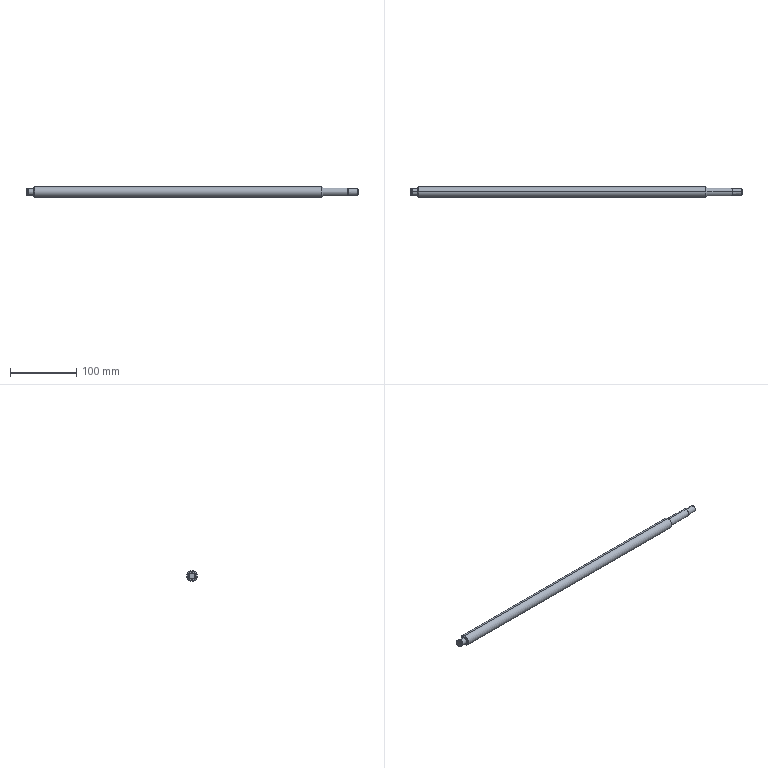Part | SolidWorks | features BaseBody 1, MoveFace 1 | 1 solid | 29 faces | box 500 x 16 x 16 mm | volume 93789 mm3 | cylinder 12 | cone 10 | plane 7 | commonest cylinder face diameters 10 x6 9.6 x2 12 x2 16 x2
STEP:
#1=CARTESIAN_POINT('',(445.773,8.,0.));
#2=VERTEX_POINT('',#1);
#3=CARTESIAN_POINT('',(445.773,0.,-8.));
#4=VERTEX_POINT('',#3);
#5=CARTESIAN_POINT('',(445.773,0.,0.));
#6=DIRECTION('',(-1.,0.,0.));
#7=DIRECTION('',(0.,0.,1.));
#8=AXIS2_PLACEMENT_3D('',#5,#6,#7);
#9=CIRCLE('',#8,8.);
#10=EDGE_CURVE('',#2,#4,#9,.T.);
#11=ORIENTED_EDGE('',*,*,#10,.T.);
#12=CARTESIAN_POINT('',(13.227,0.,-8.));
#13=VERTEX_POINT('',#12);
#14=CARTESIAN_POINT('',(500.,0.,-8.));
#15=DIRECTION('',(-1.,0.,0.));
#16=VECTOR('',#15,1000.);
#17=LINE('',#14,#16);
#18=EDGE_CURVE('',#4,#13,#17,.T.);
#19=ORIENTED_EDGE('',*,*,#18,.T.);
#20=CARTESIAN_POINT('',(13.227,8.,0.));
#21=VERTEX_POINT('',#20);
#22=CARTESIAN_POINT('',(13.227,0.,0.));
#23=DIRECTION('',(1.,0.,0.));
#24=DIRECTION('',(0.,0.,1.));
#25=AXIS2_PLACEMENT_3D('',#22,#23,#24);
#26=CIRCLE('',#25,8.);
#27=EDGE_CURVE('',#13,#21,#26,.T.);
#28=ORIENTED_EDGE('',*,*,#27,.T.);
#29=CARTESIAN_POINT('',(13.227,0.,8.));
#30=VERTEX_POINT('',#29);
#31=CARTESIAN_POINT('',(13.227,0.,0.));
#32=DIRECTION('',(1.,0.,0.));
#33=DIRECTION('',(0.,0.,1.));
#34=AXIS2_PLACEMENT_3D('',#31,#32,#33);
#35=CIRCLE('',#34,8.);
#36=EDGE_CURVE('',#21,#30,#35,.T.);
#37=ORIENTED_EDGE('',*,*,#36,.T.);
#38=CARTESIAN_POINT('',(445.773,0.,8.));
#39=VERTEX_POINT('',#38);
#40=CARTESIAN_POINT('',(500.,0.,8.));
#41=DIRECTION('',(-1.,0.,0.));
#42=VECTOR('',#41,1000.);
#43=LINE('',#40,#42);
#44=EDGE_CURVE('',#39,#30,#43,.T.);
#45=ORIENTED_EDGE('',*,*,#44,.F.);
#46=CARTESIAN_POINT('',(445.773,0.,0.));
#47=DIRECTION('',(-1.,0.,0.));
#48=DIRECTION('',(0.,0.,1.));
#49=AXIS2_PLACEMENT_3D('',#46,#47,#48);
#50=CIRCLE('',#49,8.);
#51=EDGE_CURVE('',#39,#2,#50,.T.);
#52=ORIENTED_EDGE('',*,*,#51,.T.);
#53=EDGE_LOOP('',(#11,#19,#28,#37,#45,#52));
#54=FACE_OUTER_BOUND('',#53,.T.);
#55=CARTESIAN_POINT('',(500.,0.,0.));
#56=DIRECTION('',(-1.,0.,0.));
#57=DIRECTION('',(0.,0.,1.));
#58=AXIS2_PLACEMENT_3D('',#55,#56,#57);
#59=CYLINDRICAL_SURFACE('',#58,8.);
#60=ADVANCED_FACE('',(#54),#59,.T.);
#61=CARTESIAN_POINT('',(12.,6.773,0.));
#62=VERTEX_POINT('',#61);
#63=CARTESIAN_POINT('',(12.,-6.773,0.));
#64=VERTEX_POINT('',#63);
#65=CARTESIAN_POINT('',(12.,0.,0.));
#66=DIRECTION('',(1.,0.,0.));
#67=DIRECTION('',(0.,1.,0.));
#68=AXIS2_PLACEMENT_3D('',#65,#66,#67);
#69=CIRCLE('',#68,6.773);
#70=EDGE_CURVE('',#62,#64,#69,.T.);
#71=ORIENTED_EDGE('',*,*,#70,.T.);
#72=CARTESIAN_POINT('',(13.227,-8.,0.));
#73=VERTEX_POINT('',#72);
#74=CARTESIAN_POINT('',(13.227,-8.,0.));
#75=DIRECTION('',(0.7071,-0.7071,0.));
#76=VECTOR('',#75,1000.);
#77=LINE('',#74,#76);
#78=EDGE_CURVE('',#64,#73,#77,.T.);
#79=ORIENTED_EDGE('',*,*,#78,.T.);
#80=CARTESIAN_POINT('',(13.227,0.,0.));
#81=DIRECTION('',(1.,0.,0.));
#82=DIRECTION('',(0.,0.,1.));
#83=AXIS2_PLACEMENT_3D('',#80,#81,#82);
#84=CIRCLE('',#83,8.);
#85=EDGE_CURVE('',#30,#73,#84,.T.);
#86=ORIENTED_EDGE('',*,*,#85,.F.);
#87=ORIENTED_EDGE('',*,*,#36,.F.);
#88=CARTESIAN_POINT('',(13.227,8.,0.));
#89=DIRECTION('',(0.7071,0.7071,0.));
#90=VECTOR('',#89,1000.);
#91=LINE('',#88,#90);
#92=EDGE_CURVE('',#62,#21,#91,.T.);
#93=ORIENTED_EDGE('',*,*,#92,.F.);
#94=EDGE_LOOP('',(#71,#79,#86,#87,#93));
#95=FACE_OUTER_BOUND('',#94,.T.);
#96=CARTESIAN_POINT('',(13.227,0.,0.));
#97=DIRECTION('',(1.,0.,0.));
#98=DIRECTION('',(0.,1.,0.));
#99=AXIS2_PLACEMENT_3D('',#96,#97,#98);
#100=CONICAL_SURFACE('',#99,8.,0.7854);
#101=ADVANCED_FACE('',(#95),#100,.T.);
#102=CARTESIAN_POINT('',(447.,-6.773,0.));
#103=VERTEX_POINT('',#102);
#104=CARTESIAN_POINT('',(447.,6.773,0.));
#105=VERTEX_POINT('',#104);
#106=CARTESIAN_POINT('',(447.,0.,0.));
#107=DIRECTION('',(-1.,0.,0.));
#108=DIRECTION('',(0.,-1.,0.));
#109=AXIS2_PLACEMENT_3D('',#106,#107,#108);
#110=CIRCLE('',#109,6.773);
#111=EDGE_CURVE('',#103,#105,#110,.T.);
#112=ORIENTED_EDGE('',*,*,#111,.T.);
#113=CARTESIAN_POINT('',(445.773,8.,0.));
#114=DIRECTION('',(-0.7071,0.7071,0.));
#115=VECTOR('',#114,1000.);
#116=LINE('',#113,#115);
#117=EDGE_CURVE('',#105,#2,#116,.T.);
#118=ORIENTED_EDGE('',*,*,#117,.T.);
#119=ORIENTED_EDGE('',*,*,#51,.F.);
#120=CARTESIAN_POINT('',(445.773,-8.,0.));
#121=VERTEX_POINT('',#120);
#122=CARTESIAN_POINT('',(445.773,0.,0.));
#123=DIRECTION('',(-1.,0.,0.));
#124=DIRECTION('',(0.,0.,1.));
#125=AXIS2_PLACEMENT_3D('',#122,#123,#124);
#126=CIRCLE('',#125,8.);
#127=EDGE_CURVE('',#121,#39,#126,.T.);
#128=ORIENTED_EDGE('',*,*,#127,.F.);
#129=CARTESIAN_POINT('',(445.773,-8.,0.));
#130=DIRECTION('',(-0.7071,-0.7071,0.));
#131=VECTOR('',#130,1000.);
#132=LINE('',#129,#131);
#133=EDGE_CURVE('',#103,#121,#132,.T.);
#134=ORIENTED_EDGE('',*,*,#133,.F.);
#135=EDGE_LOOP('',(#112,#118,#119,#128,#134));
#136=FACE_OUTER_BOUND('',#135,.T.);
#137=CARTESIAN_POINT('',(445.773,0.,0.));
#138=DIRECTION('',(-1.,0.,0.));
#139=DIRECTION('',(0.,-1.,0.));
#140=AXIS2_PLACEMENT_3D('',#137,#138,#139);
#141=CONICAL_SURFACE('',#140,8.,0.7854);
#142=ADVANCED_FACE('',(#136),#141,.T.);
#143=CARTESIAN_POINT('',(12.,0.,5.));
#144=VERTEX_POINT('',#143);
#145=CARTESIAN_POINT('',(12.,0.,-5.));
#146=VERTEX_POINT('',#145);
#147=CARTESIAN_POINT('',(12.,0.,0.));
#148=DIRECTION('',(-1.,0.,0.));
#149=DIRECTION('',(0.,0.,1.));
#150=AXIS2_PLACEMENT_3D('',#147,#148,#149);
#151=CIRCLE('',#150,5.);
#152=EDGE_CURVE('',#144,#146,#151,.T.);
#153=ORIENTED_EDGE('',*,*,#152,.T.);
#154=CARTESIAN_POINT('',(4.,0.,-5.));
#155=VERTEX_POINT('',#154);
#156=CARTESIAN_POINT('',(500.,0.,-5.));
#157=DIRECTION('',(-1.,0.,0.));
#158=VECTOR('',#157,1000.);
#159=LINE('',#156,#158);
#160=EDGE_CURVE('',#146,#155,#159,.T.);
#161=ORIENTED_EDGE('',*,*,#160,.T.);
#162=CARTESIAN_POINT('',(4.,0.,5.));
#163=VERTEX_POINT('',#162);
#164=CARTESIAN_POINT('',(4.,0.,0.));
#165=DIRECTION('',(1.,0.,0.));
#166=DIRECTION('',(0.,0.,1.));
#167=AXIS2_PLACEMENT_3D('',#164,#165,#166);
#168=CIRCLE('',#167,5.);
#169=EDGE_CURVE('',#155,#163,#168,.T.);
#170=ORIENTED_EDGE('',*,*,#169,.T.);
#171=CARTESIAN_POINT('',(500.,0.,5.));
#172=DIRECTION('',(-1.,0.,0.));
#173=VECTOR('',#172,1000.);
#174=LINE('',#171,#173);
#175=EDGE_CURVE('',#144,#163,#174,.T.);
#176=ORIENTED_EDGE('',*,*,#175,.F.);
#177=EDGE_LOOP('',(#153,#161,#170,#176));
#178=FACE_OUTER_BOUND('',#177,.T.);
#179=CARTESIAN_POINT('',(500.,0.,0.));
#180=DIRECTION('',(-1.,0.,0.));
#181=DIRECTION('',(0.,0.,1.));
#182=AXIS2_PLACEMENT_3D('',#179,#180,#181);
#183=CYLINDRICAL_SURFACE('',#182,5.);
#184=ADVANCED_FACE('',(#178),#183,.T.);
#185=CARTESIAN_POINT('',(484.5,0.,6.));
#186=VERTEX_POINT('',#185);
#187=CARTESIAN_POINT('',(484.5,0.,-6.));
#188=VERTEX_POINT('',#187);
#189=CARTESIAN_POINT('',(484.5,0.,0.));
#190=DIRECTION('',(-1.,0.,0.));
#191=DIRECTION('',(0.,0.,1.));
#192=AXIS2_PLACEMENT_3D('',#189,#190,#191);
#193=CIRCLE('',#192,6.);
#194=EDGE_CURVE('',#186,#188,#193,.T.);
#195=ORIENTED_EDGE('',*,*,#194,.T.);
#196=CARTESIAN_POINT('',(447.,0.,-6.));
#197=VERTEX_POINT('',#196);
#198=CARTESIAN_POINT('',(500.,0.,-6.));
#199=DIRECTION('',(-1.,0.,0.));
#200=VECTOR('',#199,1000.);
#201=LINE('',#198,#200);
#202=EDGE_CURVE('',#188,#197,#201,.T.);
#203=ORIENTED_EDGE('',*,*,#202,.T.);
#204=CARTESIAN_POINT('',(447.,0.,6.));
#205=VERTEX_POINT('',#204);
#206=CARTESIAN_POINT('',(447.,0.,0.));
#207=DIRECTION('',(1.,0.,0.));
#208=DIRECTION('',(0.,0.,1.));
#209=AXIS2_PLACEMENT_3D('',#206,#207,#208);
#210=CIRCLE('',#209,6.);
#211=EDGE_CURVE('',#197,#205,#210,.T.);
#212=ORIENTED_EDGE('',*,*,#211,.T.);
#213=CARTESIAN_POINT('',(500.,0.,6.));
#214=DIRECTION('',(-1.,0.,0.));
#215=VECTOR('',#214,1000.);
#216=LINE('',#213,#215);
#217=EDGE_CURVE('',#186,#205,#216,.T.);
#218=ORIENTED_EDGE('',*,*,#217,.F.);
#219=EDGE_LOOP('',(#195,#203,#212,#218));
#220=FACE_OUTER_BOUND('',#219,.T.);
#221=CARTESIAN_POINT('',(500.,0.,0.));
#222=DIRECTION('',(-1.,0.,0.));
#223=DIRECTION('',(0.,0.,1.));
#224=AXIS2_PLACEMENT_3D('',#221,#222,#223);
#225=CYLINDRICAL_SURFACE('',#224,6.);
#226=ADVANCED_FACE('',(#220),#225,.T.);
#227=CARTESIAN_POINT('',(485.,0.,5.5));
#228=VERTEX_POINT('',#227);
#229=CARTESIAN_POINT('',(485.,0.,-5.5));
#230=VERTEX_POINT('',#229);
#231=CARTESIAN_POINT('',(485.,0.,0.));
#232=DIRECTION('',(-1.,0.,0.));
#233=DIRECTION('',(0.,0.,1.));
#234=AXIS2_PLACEMENT_3D('',#231,#232,#233);
#235=CIRCLE('',#234,5.5);
#236=EDGE_CURVE('',#228,#230,#235,.T.);
#237=ORIENTED_EDGE('',*,*,#236,.T.);
#238=CARTESIAN_POINT('',(484.5,0.,-6.));
#239=DIRECTION('',(-0.7071,0.,-0.7071));
#240=VECTOR('',#239,1000.);
#241=LINE('',#238,#240);
#242=EDGE_CURVE('',#230,#188,#241,.T.);
#243=ORIENTED_EDGE('',*,*,#242,.T.);
#244=ORIENTED_EDGE('',*,*,#194,.F.);
#245=CARTESIAN_POINT('',(484.5,0.,6.));
#246=DIRECTION('',(-0.7071,0.,0.7071));
#247=VECTOR('',#246,1000.);
#248=LINE('',#245,#247);
#249=EDGE_CURVE('',#228,#186,#248,.T.);
#250=ORIENTED_EDGE('',*,*,#249,.F.);
#251=EDGE_LOOP('',(#237,#243,#244,#250));
#252=FACE_OUTER_BOUND('',#251,.T.);
#253=CARTESIAN_POINT('',(484.5,0.,0.));
#254=DIRECTION('',(-1.,0.,0.));
#255=DIRECTION('',(0.,0.,1.));
#256=AXIS2_PLACEMENT_3D('',#253,#254,#255);
#257=CONICAL_SURFACE('',#256,6.,0.7854);
#258=ADVANCED_FACE('',(#252),#257,.T.);
#259=CARTESIAN_POINT('',(4.,0.,4.8));
#260=VERTEX_POINT('',#259);
#261=CARTESIAN_POINT('',(4.,0.,-4.8));
#262=VERTEX_POINT('',#261);
#263=CARTESIAN_POINT('',(4.,0.,0.));
#264=DIRECTION('',(-1.,0.,0.));
#265=DIRECTION('',(0.,0.,1.));
#266=AXIS2_PLACEMENT_3D('',#263,#264,#265);
#267=CIRCLE('',#266,4.8);
#268=EDGE_CURVE('',#260,#262,#267,.T.);
#269=ORIENTED_EDGE('',*,*,#268,.T.);
#270=CARTESIAN_POINT('',(2.85,0.,-4.8));
#271=VERTEX_POINT('',#270);
#272=CARTESIAN_POINT('',(500.,0.,-4.8));
#273=DIRECTION('',(-1.,0.,0.));
#274=VECTOR('',#273,1000.);
#275=LINE('',#272,#274);
#276=EDGE_CURVE('',#262,#271,#275,.T.);
#277=ORIENTED_EDGE('',*,*,#276,.T.);
#278=CARTESIAN_POINT('',(2.85,0.,4.8));
#279=VERTEX_POINT('',#278);
#280=CARTESIAN_POINT('',(2.85,0.,0.));
#281=DIRECTION('',(1.,0.,0.));
#282=DIRECTION('',(0.,0.,1.));
#283=AXIS2_PLACEMENT_3D('',#280,#281,#282);
#284=CIRCLE('',#283,4.8);
#285=EDGE_CURVE('',#271,#279,#284,.T.);
#286=ORIENTED_EDGE('',*,*,#285,.T.);
#287=CARTESIAN_POINT('',(500.,0.,4.8));
#288=DIRECTION('',(-1.,0.,0.));
#289=VECTOR('',#288,1000.);
#290=LINE('',#287,#289);
#291=EDGE_CURVE('',#260,#279,#290,.T.);
#292=ORIENTED_EDGE('',*,*,#291,.F.);
#293=EDGE_LOOP('',(#269,#277,#286,#292));
#294=FACE_OUTER_BOUND('',#293,.T.);
#295=CARTESIAN_POINT('',(500.,0.,0.));
#296=DIRECTION('',(-1.,0.,0.));
#297=DIRECTION('',(0.,0.,1.));
#298=AXIS2_PLACEMENT_3D('',#295,#296,#297);
#299=CYLINDRICAL_SURFACE('',#298,4.8);
#300=ADVANCED_FACE('',(#294),#299,.T.);
#301=CARTESIAN_POINT('',(499.5,5.,0.));
#302=VERTEX_POINT('',#301);
#303=CARTESIAN_POINT('',(499.5,0.,-5.));
#304=VERTEX_POINT('',#303);
#305=CARTESIAN_POINT('',(499.5,0.,0.));
#306=DIRECTION('',(-1.,0.,0.));
#307=DIRECTION('',(0.,0.,1.));
#308=AXIS2_PLACEMENT_3D('',#305,#306,#307);
#309=CIRCLE('',#308,5.);
#310=EDGE_CURVE('',#302,#304,#309,.T.);
#311=ORIENTED_EDGE('',*,*,#310,.T.);
#312=CARTESIAN_POINT('',(485.,0.,-5.));
#313=VERTEX_POINT('',#312);
#314=CARTESIAN_POINT('',(500.,0.,-5.));
#315=DIRECTION('',(-1.,0.,0.));
#316=VECTOR('',#315,1000.);
#317=LINE('',#314,#316);
#318=EDGE_CURVE('',#304,#313,#317,.T.);
#319=ORIENTED_EDGE('',*,*,#318,.T.);
#320=CARTESIAN_POINT('',(485.,0.,5.));
#321=VERTEX_POINT('',#320);
#322=CARTESIAN_POINT('',(485.,0.,0.));
#323=DIRECTION('',(1.,0.,0.));
#324=DIRECTION('',(0.,0.,1.));
#325=AXIS2_PLACEMENT_3D('',#322,#323,#324);
#326=CIRCLE('',#325,5.);
#327=EDGE_CURVE('',#313,#321,#326,.T.);
#328=ORIENTED_EDGE('',*,*,#327,.T.);
#329=CARTESIAN_POINT('',(499.5,0.,5.));
#330=VERTEX_POINT('',#329);
#331=CARTESIAN_POINT('',(500.,0.,5.));
#332=DIRECTION('',(-1.,0.,0.));
#333=VECTOR('',#332,1000.);
#334=LINE('',#331,#333);
#335=EDGE_CURVE('',#330,#321,#334,.T.);
#336=ORIENTED_EDGE('',*,*,#335,.F.);
#337=CARTESIAN_POINT('',(499.5,0.,0.));
#338=DIRECTION('',(-1.,0.,0.));
#339=DIRECTION('',(0.,0.,1.));
#340=AXIS2_PLACEMENT_3D('',#337,#338,#339);
#341=CIRCLE('',#340,5.);
#342=EDGE_CURVE('',#330,#302,#341,.T.);
#343=ORIENTED_EDGE('',*,*,#342,.T.);
#344=EDGE_LOOP('',(#311,#319,#328,#336,#343));
#345=FACE_OUTER_BOUND('',#344,.T.);
#346=CARTESIAN_POINT('',(500.,0.,0.));
#347=DIRECTION('',(-1.,0.,0.));
#348=DIRECTION('',(0.,0.,1.));
#349=AXIS2_PLACEMENT_3D('',#346,#347,#348);
#350=CYLINDRICAL_SURFACE('',#349,5.);
#351=ADVANCED_FACE('',(#345),#350,.T.);
#352=CARTESIAN_POINT('',(2.85,0.,5.));
#353=VERTEX_POINT('',#352);
#354=CARTESIAN_POINT('',(2.85,0.,-5.));
#355=VERTEX_POINT('',#354);
#356=CARTESIAN_POINT('',(2.85,0.,0.));
#357=DIRECTION('',(-1.,0.,0.));
#358=DIRECTION('',(0.,0.,1.));
#359=AXIS2_PLACEMENT_3D('',#356,#357,#358);
#360=CIRCLE('',#359,5.);
#361=EDGE_CURVE('',#353,#355,#360,.T.);
#362=ORIENTED_EDGE('',*,*,#361,.T.);
#363=CARTESIAN_POINT('',(0.5,0.,-5.));
#364=VERTEX_POINT('',#363);
#365=CARTESIAN_POINT('',(500.,0.,-5.));
#366=DIRECTION('',(-1.,0.,0.));
#367=VECTOR('',#366,1000.);
#368=LINE('',#365,#367);
#369=EDGE_CURVE('',#355,#364,#368,.T.);
#370=ORIENTED_EDGE('',*,*,#369,.T.);
#371=CARTESIAN_POINT('',(0.5,0.,5.));
#372=VERTEX_POINT('',#371);
#373=CARTESIAN_POINT('',(0.5,0.,0.));
#374=DIRECTION('',(1.,0.,0.));
#375=DIRECTION('',(0.,0.,1.));
#376=AXIS2_PLACEMENT_3D('',#373,#374,#375);
#377=CIRCLE('',#376,5.);
#378=EDGE_CURVE('',#364,#372,#377,.T.);
#379=ORIENTED_EDGE('',*,*,#378,.T.);
#380=CARTESIAN_POINT('',(500.,0.,5.));
#381=DIRECTION('',(-1.,0.,0.));
#382=VECTOR('',#381,1000.);
#383=LINE('',#380,#382);
#384=EDGE_CURVE('',#353,#372,#383,.T.);
#385=ORIENTED_EDGE('',*,*,#384,.F.);
#386=EDGE_LOOP('',(#362,#370,#379,#385));
#387=FACE_OUTER_BOUND('',#386,.T.);
#388=CARTESIAN_POINT('',(500.,0.,0.));
#389=DIRECTION('',(-1.,0.,0.));
#390=DIRECTION('',(0.,0.,1.));
#391=AXIS2_PLACEMENT_3D('',#388,#389,#390);
#392=CYLINDRICAL_SURFACE('',#391,5.);
#393=ADVANCED_FACE('',(#387),#392,.T.);
#394=CARTESIAN_POINT('',(500.,-4.5,0.));
#395=VERTEX_POINT('',#394);
#396=CARTESIAN_POINT('',(500.,4.5,0.));
#397=VERTEX_POINT('',#396);
#398=CARTESIAN_POINT('',(500.,0.,0.));
#399=DIRECTION('',(-1.,0.,0.));
#400=DIRECTION('',(0.,-1.,0.));
#401=AXIS2_PLACEMENT_3D('',#398,#399,#400);
#402=CIRCLE('',#401,4.5);
#403=EDGE_CURVE('',#395,#397,#402,.T.);
#404=ORIENTED_EDGE('',*,*,#403,.T.);
#405=CARTESIAN_POINT('',(499.5,5.,0.));
#406=DIRECTION('',(-0.7071,0.7071,0.));
#407=VECTOR('',#406,1000.);
#408=LINE('',#405,#407);
#409=EDGE_CURVE('',#397,#302,#408,.T.);
#410=ORIENTED_EDGE('',*,*,#409,.T.);
#411=ORIENTED_EDGE('',*,*,#342,.F.);
#412=CARTESIAN_POINT('',(499.5,-5.,0.));
#413=VERTEX_POINT('',#412);
#414=CARTESIAN_POINT('',(499.5,0.,0.));
#415=DIRECTION('',(-1.,0.,0.));
#416=DIRECTION('',(0.,0.,1.));
#417=AXIS2_PLACEMENT_3D('',#414,#415,#416);
#418=CIRCLE('',#417,5.);
#419=EDGE_CURVE('',#413,#330,#418,.T.);
#420=ORIENTED_EDGE('',*,*,#419,.F.);
#421=CARTESIAN_POINT('',(499.5,-5.,0.));
#422=DIRECTION('',(-0.7071,-0.7071,0.));
#423=VECTOR('',#422,1000.);
#424=LINE('',#421,#423);
#425=EDGE_CURVE('',#395,#413,#424,.T.);
#426=ORIENTED_EDGE('',*,*,#425,.F.);
#427=EDGE_LOOP('',(#404,#410,#411,#420,#426));
#428=FACE_OUTER_BOUND('',#427,.T.);
#429=CARTESIAN_POINT('',(499.5,0.,0.));
#430=DIRECTION('',(-1.,0.,0.));
#431=DIRECTION('',(0.,-1.,0.));
#432=AXIS2_PLACEMENT_3D('',#429,#430,#431);
#433=CONICAL_SURFACE('',#432,5.,0.7854);
#434=ADVANCED_FACE('',(#428),#433,.T.);
#435=CARTESIAN_POINT('',(0.,0.,-4.5));
#436=VERTEX_POINT('',#435);
#437=CARTESIAN_POINT('',(0.,0.,4.5));
#438=VERTEX_POINT('',#437);
#439=CARTESIAN_POINT('',(0.,0.,0.));
#440=DIRECTION('',(1.,0.,0.));
#441=DIRECTION('',(0.,0.,-1.));
#442=AXIS2_PLACEMENT_3D('',#439,#440,#441);
#443=CIRCLE('',#442,4.5);
#444=EDGE_CURVE('',#436,#438,#443,.T.);
#445=ORIENTED_EDGE('',*,*,#444,.T.);
#446=CARTESIAN_POINT('',(0.5,0.,5.));
#447=DIRECTION('',(0.7071,0.,0.7071));
#448=VECTOR('',#447,1000.);
#449=LINE('',#446,#448);
#450=EDGE_CURVE('',#438,#372,#449,.T.);
#451=ORIENTED_EDGE('',*,*,#450,.T.);
#452=ORIENTED_EDGE('',*,*,#378,.F.);
#453=CARTESIAN_POINT('',(0.5,0.,-5.));
#454=DIRECTION('',(0.7071,0.,-0.7071));
#455=VECTOR('',#454,1000.);
#456=LINE('',#453,#455);
#457=EDGE_CURVE('',#436,#364,#456,.T.);
#458=ORIENTED_EDGE('',*,*,#457,.F.);
#459=EDGE_LOOP('',(#445,#451,#452,#458));
#460=FACE_OUTER_BOUND('',#459,.T.);
#461=CARTESIAN_POINT('',(0.5,0.,0.));
#462=DIRECTION('',(1.,0.,0.));
#463=DIRECTION('',(0.,0.,-1.));
#464=AXIS2_PLACEMENT_3D('',#461,#462,#463);
#465=CONICAL_SURFACE('',#464,5.,0.7854);
#466=ADVANCED_FACE('',(#460),#465,.T.);
#467=ORIENTED_EDGE('',*,*,#18,.F.);
#468=CARTESIAN_POINT('',(445.773,0.,0.));
#469=DIRECTION('',(-1.,0.,0.));
#470=DIRECTION('',(0.,0.,1.));
#471=AXIS2_PLACEMENT_3D('',#468,#469,#470);
#472=CIRCLE('',#471,8.);
#473=EDGE_CURVE('',#4,#121,#472,.T.);
#474=ORIENTED_EDGE('',*,*,#473,.T.);
#475=ORIENTED_EDGE('',*,*,#127,.T.);
#476=ORIENTED_EDGE('',*,*,#44,.T.);
#477=ORIENTED_EDGE('',*,*,#85,.T.);
#478=CARTESIAN_POINT('',(13.227,0.,0.));
#479=DIRECTION('',(1.,0.,0.));
#480=DIRECTION('',(0.,0.,1.));
#481=AXIS2_PLACEMENT_3D('',#478,#479,#480);
#482=CIRCLE('',#481,8.);
#483=EDGE_CURVE('',#73,#13,#482,.T.);
#484=ORIENTED_EDGE('',*,*,#483,.T.);
#485=EDGE_LOOP('',(#467,#474,#475,#476,#477,#484));
#486=FACE_OUTER_BOUND('',#485,.T.);
#487=CARTESIAN_POINT('',(500.,0.,0.));
#488=DIRECTION('',(-1.,0.,0.));
#489=DIRECTION('',(0.,0.,1.));
#490=AXIS2_PLACEMENT_3D('',#487,#488,#489);
#491=CYLINDRICAL_SURFACE('',#490,8.);
#492=ADVANCED_FACE('',(#486),#491,.T.);
#493=ORIENTED_EDGE('',*,*,#78,.F.);
#494=CARTESIAN_POINT('',(12.,0.,0.));
#495=DIRECTION('',(1.,0.,0.));
#496=DIRECTION('',(0.,1.,0.));
#497=AXIS2_PLACEMENT_3D('',#494,#495,#496);
#498=CIRCLE('',#497,6.773);
#499=EDGE_CURVE('',#64,#62,#498,.T.);
#500=ORIENTED_EDGE('',*,*,#499,.T.);
#501=ORIENTED_EDGE('',*,*,#92,.T.);
#502=ORIENTED_EDGE('',*,*,#27,.F.);
#503=ORIENTED_EDGE('',*,*,#483,.F.);
#504=EDGE_LOOP('',(#493,#500,#501,#502,#503));
#505=FACE_OUTER_BOUND('',#504,.T.);
#506=CARTESIAN_POINT('',(13.227,0.,0.));
#507=DIRECTION('',(1.,0.,0.));
#508=DIRECTION('',(0.,1.,0.));
#509=AXIS2_PLACEMENT_3D('',#506,#507,#508);
#510=CONICAL_SURFACE('',#509,8.,0.7854);
#511=ADVANCED_FACE('',(#505),#510,.T.);
#512=ORIENTED_EDGE('',*,*,#117,.F.);
#513=CARTESIAN_POINT('',(447.,0.,0.));
#514=DIRECTION('',(-1.,0.,0.));
#515=DIRECTION('',(0.,-1.,0.));
#516=AXIS2_PLACEMENT_3D('',#513,#514,#515);
#517=CIRCLE('',#516,6.773);
#518=EDGE_CURVE('',#105,#103,#517,.T.);
#519=ORIENTED_EDGE('',*,*,#518,.T.);
#520=ORIENTED_EDGE('',*,*,#133,.T.);
#521=ORIENTED_EDGE('',*,*,#473,.F.);
#522=ORIENTED_EDGE('',*,*,#10,.F.);
#523=EDGE_LOOP('',(#512,#519,#520,#521,#522));
#524=FACE_OUTER_BOUND('',#523,.T.);
#525=CARTESIAN_POINT('',(445.773,0.,0.));
#526=DIRECTION('',(-1.,0.,0.));
#527=DIRECTION('',(0.,-1.,0.));
#528=AXIS2_PLACEMENT_3D('',#525,#526,#527);
#529=CONICAL_SURFACE('',#528,8.,0.7854);
#530=ADVANCED_FACE('',(#524),#529,.T.);
#531=ORIENTED_EDGE('',*,*,#152,.F.);
#532=CARTESIAN_POINT('',(12.,0.,0.));
#533=DIRECTION('',(-1.,0.,0.));
#534=DIRECTION('',(0.,0.,1.));
#535=AXIS2_PLACEMENT_3D('',#532,#533,#534);
#536=CIRCLE('',#535,5.);
#537=EDGE_CURVE('',#146,#144,#536,.T.);
#538=ORIENTED_EDGE('',*,*,#537,.F.);
#539=EDGE_LOOP('',(#531,#538));
#540=FACE_BOUND('',#539,.T.);
#541=ORIENTED_EDGE('',*,*,#70,.F.);
#542=ORIENTED_EDGE('',*,*,#499,.F.);
#543=EDGE_LOOP('',(#541,#542));
#544=FACE_OUTER_BOUND('',#543,.T.);
#545=CARTESIAN_POINT('',(12.,5.,0.));
#546=DIRECTION('',(1.,0.,0.));
#547=DIRECTION('',(0.,0.,-1.));
#548=AXIS2_PLACEMENT_3D('',#545,#546,#547);
#549=PLANE('',#548);
#550=ADVANCED_FACE('',(#540,#544),#549,.F.);
#551=ORIENTED_EDGE('',*,*,#111,.F.);
#552=ORIENTED_EDGE('',*,*,#518,.F.);
#553=EDGE_LOOP('',(#551,#552));
#554=FACE_OUTER_BOUND('',#553,.T.);
#555=CARTESIAN_POINT('',(447.,0.,0.));
#556=DIRECTION('',(1.,0.,0.));
#557=DIRECTION('',(0.,0.,1.));
#558=AXIS2_PLACEMENT_3D('',#555,#556,#557);
#559=CIRCLE('',#558,6.);
#560=EDGE_CURVE('',#205,#197,#559,.T.);
#561=ORIENTED_EDGE('',*,*,#560,.F.);
#562=ORIENTED_EDGE('',*,*,#211,.F.);
#563=EDGE_LOOP('',(#561,#562));
#564=FACE_BOUND('',#563,.T.);
#565=CARTESIAN_POINT('',(447.,6.773,0.));
#566=DIRECTION('',(-1.,0.,0.));
#567=DIRECTION('',(0.,0.,1.));
#568=AXIS2_PLACEMENT_3D('',#565,#566,#567);
#569=PLANE('',#568);
#570=ADVANCED_FACE('',(#554,#564),#569,.F.);
#571=ORIENTED_EDGE('',*,*,#160,.F.);
#572=ORIENTED_EDGE('',*,*,#537,.T.);
#573=ORIENTED_EDGE('',*,*,#175,.T.);
#574=CARTESIAN_POINT('',(4.,0.,0.));
#575=DIRECTION('',(1.,0.,0.));
#576=DIRECTION('',(0.,0.,1.));
#577=AXIS2_PLACEMENT_3D('',#574,#575,#576);
#578=CIRCLE('',#577,5.);
#579=EDGE_CURVE('',#163,#155,#578,.T.);
#580=ORIENTED_EDGE('',*,*,#579,.T.);
#581=EDGE_LOOP('',(#571,#572,#573,#580));
#582=FACE_OUTER_BOUND('',#581,.T.);
#583=CARTESIAN_POINT('',(500.,0.,0.));
#584=DIRECTION('',(-1.,0.,0.));
#585=DIRECTION('',(0.,0.,1.));
#586=AXIS2_PLACEMENT_3D('',#583,#584,#585);
#587=CYLINDRICAL_SURFACE('',#586,5.);
#588=ADVANCED_FACE('',(#582),#587,.T.);
#589=ORIENTED_EDGE('',*,*,#202,.F.);
#590=CARTESIAN_POINT('',(484.5,0.,0.));
#591=DIRECTION('',(-1.,0.,0.));
#592=DIRECTION('',(0.,0.,1.));
#593=AXIS2_PLACEMENT_3D('',#590,#591,#592);
#594=CIRCLE('',#593,6.);
#595=EDGE_CURVE('',#188,#186,#594,.T.);
#596=ORIENTED_EDGE('',*,*,#595,.T.);
#597=ORIENTED_EDGE('',*,*,#217,.T.);
#598=ORIENTED_EDGE('',*,*,#560,.T.);
#599=EDGE_LOOP('',(#589,#596,#597,#598));
#600=FACE_OUTER_BOUND('',#599,.T.);
#601=CARTESIAN_POINT('',(500.,0.,0.));
#602=DIRECTION('',(-1.,0.,0.));
#603=DIRECTION('',(0.,0.,1.));
#604=AXIS2_PLACEMENT_3D('',#601,#602,#603);
#605=CYLINDRICAL_SURFACE('',#604,6.);
#606=ADVANCED_FACE('',(#600),#605,.T.);
#607=ORIENTED_EDGE('',*,*,#268,.F.);
#608=CARTESIAN_POINT('',(4.,0.,0.));
#609=DIRECTION('',(-1.,0.,0.));
#610=DIRECTION('',(0.,0.,1.));
#611=AXIS2_PLACEMENT_3D('',#608,#609,#610);
#612=CIRCLE('',#611,4.8);
#613=EDGE_CURVE('',#262,#260,#612,.T.);
#614=ORIENTED_EDGE('',*,*,#613,.F.);
#615=EDGE_LOOP('',(#607,#614));
#616=FACE_BOUND('',#615,.T.);
#617=ORIENTED_EDGE('',*,*,#579,.F.);
#618=ORIENTED_EDGE('',*,*,#169,.F.);
#619=EDGE_LOOP('',(#617,#618));
#620=FACE_OUTER_BOUND('',#619,.T.);
#621=CARTESIAN_POINT('',(4.,4.8,0.));
#622=DIRECTION('',(1.,0.,0.));
#623=DIRECTION('',(0.,0.,-1.));
#624=AXIS2_PLACEMENT_3D('',#621,#622,#623);
#625=PLANE('',#624);
#626=ADVANCED_FACE('',(#616,#620),#625,.F.);
#627=ORIENTED_EDGE('',*,*,#242,.F.);
#628=CARTESIAN_POINT('',(485.,0.,0.));
#629=DIRECTION('',(-1.,0.,0.));
#630=DIRECTION('',(0.,0.,1.));
#631=AXIS2_PLACEMENT_3D('',#628,#629,#630);
#632=CIRCLE('',#631,5.5);
#633=EDGE_CURVE('',#230,#228,#632,.T.);
#634=ORIENTED_EDGE('',*,*,#633,.T.);
#635=ORIENTED_EDGE('',*,*,#249,.T.);
#636=ORIENTED_EDGE('',*,*,#595,.F.);
#637=EDGE_LOOP('',(#627,#634,#635,#636));
#638=FACE_OUTER_BOUND('',#637,.T.);
#639=CARTESIAN_POINT('',(484.5,0.,0.));
#640=DIRECTION('',(-1.,0.,0.));
#641=DIRECTION('',(0.,0.,1.));
#642=AXIS2_PLACEMENT_3D('',#639,#640,#641);
#643=CONICAL_SURFACE('',#642,6.,0.7854);
#644=ADVANCED_FACE('',(#638),#643,.T.);
#645=ORIENTED_EDGE('',*,*,#276,.F.);
#646=ORIENTED_EDGE('',*,*,#613,.T.);
#647=ORIENTED_EDGE('',*,*,#291,.T.);
#648=CARTESIAN_POINT('',(2.85,0.,0.));
#649=DIRECTION('',(1.,0.,0.));
#650=DIRECTION('',(0.,0.,1.));
#651=AXIS2_PLACEMENT_3D('',#648,#649,#650);
#652=CIRCLE('',#651,4.8);
#653=EDGE_CURVE('',#279,#271,#652,.T.);
#654=ORIENTED_EDGE('',*,*,#653,.T.);
#655=EDGE_LOOP('',(#645,#646,#647,#654));
#656=FACE_OUTER_BOUND('',#655,.T.);
#657=CARTESIAN_POINT('',(500.,0.,0.));
#658=DIRECTION('',(-1.,0.,0.));
#659=DIRECTION('',(0.,0.,1.));
#660=AXIS2_PLACEMENT_3D('',#657,#658,#659);
#661=CYLINDRICAL_SURFACE('',#660,4.8);
#662=ADVANCED_FACE('',(#656),#661,.T.);
#663=ORIENTED_EDGE('',*,*,#236,.F.);
#664=ORIENTED_EDGE('',*,*,#633,.F.);
#665=EDGE_LOOP('',(#663,#664));
#666=FACE_OUTER_BOUND('',#665,.T.);
#667=CARTESIAN_POINT('',(485.,0.,0.));
#668=DIRECTION('',(1.,0.,0.));
#669=DIRECTION('',(0.,0.,1.));
#670=AXIS2_PLACEMENT_3D('',#667,#668,#669);
#671=CIRCLE('',#670,5.);
#672=EDGE_CURVE('',#321,#313,#671,.T.);
#673=ORIENTED_EDGE('',*,*,#672,.F.);
#674=ORIENTED_EDGE('',*,*,#327,.F.);
#675=EDGE_LOOP('',(#673,#674));
#676=FACE_BOUND('',#675,.T.);
#677=CARTESIAN_POINT('',(485.,5.5,0.));
#678=DIRECTION('',(-1.,0.,0.));
#679=DIRECTION('',(0.,0.,1.));
#680=AXIS2_PLACEMENT_3D('',#677,#678,#679);
#681=PLANE('',#680);
#682=ADVANCED_FACE('',(#666,#676),#681,.F.);
#683=ORIENTED_EDGE('',*,*,#361,.F.);
#684=CARTESIAN_POINT('',(2.85,0.,0.));
#685=DIRECTION('',(-1.,0.,0.));
#686=DIRECTION('',(0.,0.,1.));
#687=AXIS2_PLACEMENT_3D('',#684,#685,#686);
#688=CIRCLE('',#687,5.);
#689=EDGE_CURVE('',#355,#353,#688,.T.);
#690=ORIENTED_EDGE('',*,*,#689,.F.);
#691=EDGE_LOOP('',(#683,#690));
#692=FACE_OUTER_BOUND('',#691,.T.);
#693=ORIENTED_EDGE('',*,*,#653,.F.);
#694=ORIENTED_EDGE('',*,*,#285,.F.);
#695=EDGE_LOOP('',(#693,#694));
#696=FACE_BOUND('',#695,.T.);
#697=CARTESIAN_POINT('',(2.85,5.,0.));
#698=DIRECTION('',(-1.,0.,0.));
#699=DIRECTION('',(0.,0.,1.));
#700=AXIS2_PLACEMENT_3D('',#697,#698,#699);
#701=PLANE('',#700);
#702=ADVANCED_FACE('',(#692,#696),#701,.F.);
#703=ORIENTED_EDGE('',*,*,#318,.F.);
#704=CARTESIAN_POINT('',(499.5,0.,0.));
#705=DIRECTION('',(-1.,0.,0.));
#706=DIRECTION('',(0.,0.,1.));
#707=AXIS2_PLACEMENT_3D('',#704,#705,#706);
#708=CIRCLE('',#707,5.);
#709=EDGE_CURVE('',#304,#413,#708,.T.);
#710=ORIENTED_EDGE('',*,*,#709,.T.);
#711=ORIENTED_EDGE('',*,*,#419,.T.);
#712=ORIENTED_EDGE('',*,*,#335,.T.);
#713=ORIENTED_EDGE('',*,*,#672,.T.);
#714=EDGE_LOOP('',(#703,#710,#711,#712,#713));
#715=FACE_OUTER_BOUND('',#714,.T.);
#716=CARTESIAN_POINT('',(500.,0.,0.));
#717=DIRECTION('',(-1.,0.,0.));
#718=DIRECTION('',(0.,0.,1.));
#719=AXIS2_PLACEMENT_3D('',#716,#717,#718);
#720=CYLINDRICAL_SURFACE('',#719,5.);
#721=ADVANCED_FACE('',(#715),#720,.T.);
#722=ORIENTED_EDGE('',*,*,#369,.F.);
#723=ORIENTED_EDGE('',*,*,#689,.T.);
#724=ORIENTED_EDGE('',*,*,#384,.T.);
#725=CARTESIAN_POINT('',(0.5,0.,0.));
#726=DIRECTION('',(1.,0.,0.));
#727=DIRECTION('',(0.,0.,1.));
#728=AXIS2_PLACEMENT_3D('',#725,#726,#727);
#729=CIRCLE('',#728,5.);
#730=EDGE_CURVE('',#372,#364,#729,.T.);
#731=ORIENTED_EDGE('',*,*,#730,.T.);
#732=EDGE_LOOP('',(#722,#723,#724,#731));
#733=FACE_OUTER_BOUND('',#732,.T.);
#734=CARTESIAN_POINT('',(500.,0.,0.));
#735=DIRECTION('',(-1.,0.,0.));
#736=DIRECTION('',(0.,0.,1.));
#737=AXIS2_PLACEMENT_3D('',#734,#735,#736);
#738=CYLINDRICAL_SURFACE('',#737,5.);
#739=ADVANCED_FACE('',(#733),#738,.T.);
#740=ORIENTED_EDGE('',*,*,#409,.F.);
#741=CARTESIAN_POINT('',(500.,0.,0.));
#742=DIRECTION('',(-1.,0.,0.));
#743=DIRECTION('',(0.,-1.,0.));
#744=AXIS2_PLACEMENT_3D('',#741,#742,#743);
#745=CIRCLE('',#744,4.5);
#746=EDGE_CURVE('',#397,#395,#745,.T.);
#747=ORIENTED_EDGE('',*,*,#746,.T.);
#748=ORIENTED_EDGE('',*,*,#425,.T.);
#749=ORIENTED_EDGE('',*,*,#709,.F.);
#750=ORIENTED_EDGE('',*,*,#310,.F.);
#751=EDGE_LOOP('',(#740,#747,#748,#749,#750));
#752=FACE_OUTER_BOUND('',#751,.T.);
#753=CARTESIAN_POINT('',(499.5,0.,0.));
#754=DIRECTION('',(-1.,0.,0.));
#755=DIRECTION('',(0.,-1.,0.));
#756=AXIS2_PLACEMENT_3D('',#753,#754,#755);
#757=CONICAL_SURFACE('',#756,5.,0.7854);
#758=ADVANCED_FACE('',(#752),#757,.T.);
#759=ORIENTED_EDGE('',*,*,#450,.F.);
#760=CARTESIAN_POINT('',(0.,0.,0.));
#761=DIRECTION('',(1.,0.,0.));
#762=DIRECTION('',(0.,0.,-1.));
#763=AXIS2_PLACEMENT_3D('',#760,#761,#762);
#764=CIRCLE('',#763,4.5);
#765=EDGE_CURVE('',#438,#436,#764,.T.);
#766=ORIENTED_EDGE('',*,*,#765,.T.);
#767=ORIENTED_EDGE('',*,*,#457,.T.);
#768=ORIENTED_EDGE('',*,*,#730,.F.);
#769=EDGE_LOOP('',(#759,#766,#767,#768));
#770=FACE_OUTER_BOUND('',#769,.T.);
#771=CARTESIAN_POINT('',(0.5,0.,0.));
#772=DIRECTION('',(1.,0.,0.));
#773=DIRECTION('',(0.,0.,-1.));
#774=AXIS2_PLACEMENT_3D('',#771,#772,#773);
#775=CONICAL_SURFACE('',#774,5.,0.7854);
#776=ADVANCED_FACE('',(#770),#775,.T.);
#777=ORIENTED_EDGE('',*,*,#403,.F.);
#778=ORIENTED_EDGE('',*,*,#746,.F.);
#779=EDGE_LOOP('',(#777,#778));
#780=FACE_OUTER_BOUND('',#779,.T.);
#781=CARTESIAN_POINT('',(500.,4.5,0.));
#782=DIRECTION('',(-1.,0.,0.));
#783=DIRECTION('',(0.,0.,1.));
#784=AXIS2_PLACEMENT_3D('',#781,#782,#783);
#785=PLANE('',#784);
#786=ADVANCED_FACE('',(#780),#785,.F.);
#787=ORIENTED_EDGE('',*,*,#444,.F.);
#788=ORIENTED_EDGE('',*,*,#765,.F.);
#789=EDGE_LOOP('',(#787,#788));
#790=FACE_OUTER_BOUND('',#789,.T.);
#791=CARTESIAN_POINT('',(0.,0.,0.));
#792=DIRECTION('',(1.,0.,0.));
#793=DIRECTION('',(0.,0.,-1.));
#794=AXIS2_PLACEMENT_3D('',#791,#792,#793);
#795=PLANE('',#794);
#796=ADVANCED_FACE('',(#790),#795,.F.);
#797=CLOSED_SHELL('',(#60,#101,#142,#184,#226,#258,#300,#351,#393,#434,#466,#492,#511,#530,#550,#570,#588,#606,#626,#644,#662,#682,#702,#721,#739,#758,#776,#786,#796));
#798=MANIFOLD_SOLID_BREP('',#797);
#799=CARTESIAN_POINT('',(0.,0.,0.));
#800=DIRECTION('',(0.,0.,1.));
#801=DIRECTION('',(1.,0.,0.));
#802=AXIS2_PLACEMENT_3D('',#799,#800,#801);
#803=(LENGTH_UNIT()NAMED_UNIT(*)SI_UNIT(.MILLI.,.METRE.));
#804=UNCERTAINTY_MEASURE_WITH_UNIT(LENGTH_MEASURE(0.00001),#803,'','');
#805=(NAMED_UNIT(*)PLANE_ANGLE_UNIT()SI_UNIT($,.RADIAN.));
#806=(NAMED_UNIT(*)SI_UNIT($,.STERADIAN.)SOLID_ANGLE_UNIT());
#807=(GEOMETRIC_REPRESENTATION_CONTEXT(3)GLOBAL_UNCERTAINTY_ASSIGNED_CONTEXT((#804))GLOBAL_UNIT_ASSIGNED_CONTEXT((#803,#805,#806))REPRESENTATION_CONTEXT('',''));
#808=ADVANCED_BREP_SHAPE_REPRESENTATION('',(#798,#802),#807);